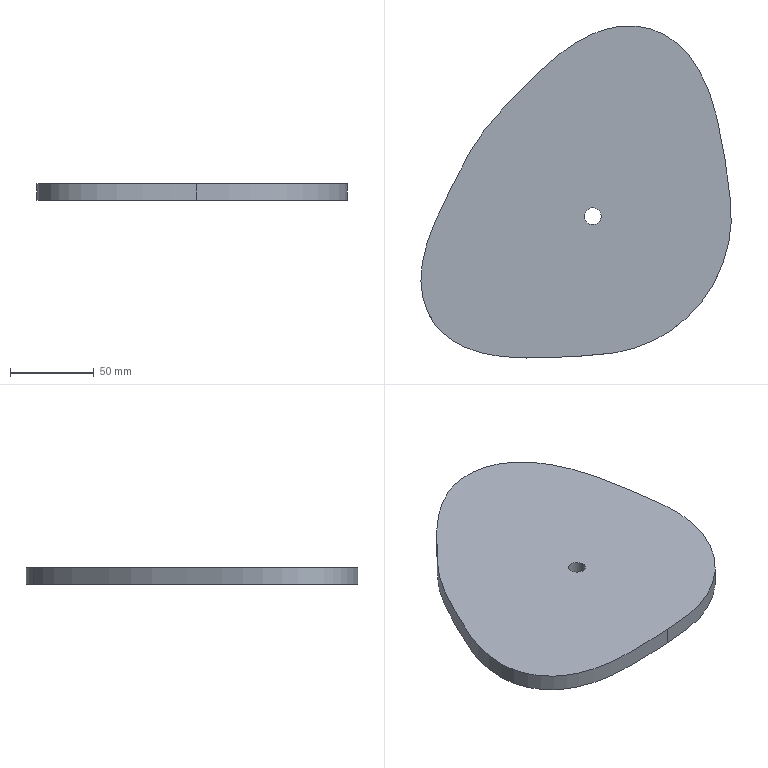Part | SolidWorks | features Extrusion 1 | 1 solid | 6 faces | box 185.51 x 198.55 x 10 mm | volume 275088 mm3 | cylinder 2 | plane 2 | spline 2 | commonest cylinder face diameters 10 x2
STEP:
#1=CARTESIAN_POINT('',(-5.,0.,10.));
#2=VERTEX_POINT('',#1);
#3=CARTESIAN_POINT('',(5.,0.,10.));
#4=VERTEX_POINT('',#3);
#5=CARTESIAN_POINT('',(0.,0.,10.));
#6=DIRECTION('',(0.,0.,1.));
#7=DIRECTION('',(1.,0.,0.));
#8=AXIS2_PLACEMENT_3D('',#5,#6,#7);
#9=CIRCLE('',#8,5.);
#10=EDGE_CURVE('',#2,#4,#9,.T.);
#11=ORIENTED_EDGE('',*,*,#10,.T.);
#12=CARTESIAN_POINT('',(5.,0.,0.));
#13=VERTEX_POINT('',#12);
#14=CARTESIAN_POINT('',(5.,0.,10.));
#15=DIRECTION('',(0.,0.,-1.));
#16=VECTOR('',#15,1000.);
#17=LINE('',#14,#16);
#18=EDGE_CURVE('',#4,#13,#17,.T.);
#19=ORIENTED_EDGE('',*,*,#18,.T.);
#20=CARTESIAN_POINT('',(-5.,0.,0.));
#21=VERTEX_POINT('',#20);
#22=CARTESIAN_POINT('',(0.,0.,0.));
#23=DIRECTION('',(0.,0.,1.));
#24=DIRECTION('',(1.,0.,0.));
#25=AXIS2_PLACEMENT_3D('',#22,#23,#24);
#26=CIRCLE('',#25,5.);
#27=EDGE_CURVE('',#21,#13,#26,.T.);
#28=ORIENTED_EDGE('',*,*,#27,.F.);
#29=CARTESIAN_POINT('',(-5.,0.,10.));
#30=DIRECTION('',(0.,0.,-1.));
#31=VECTOR('',#30,1000.);
#32=LINE('',#29,#31);
#33=EDGE_CURVE('',#2,#21,#32,.T.);
#34=ORIENTED_EDGE('',*,*,#33,.F.);
#35=EDGE_LOOP('',(#11,#19,#28,#34));
#36=FACE_OUTER_BOUND('',#35,.T.);
#37=CARTESIAN_POINT('',(0.,0.,10.));
#38=DIRECTION('',(0.,0.,-1.));
#39=DIRECTION('',(-1.,0.,0.));
#40=AXIS2_PLACEMENT_3D('',#37,#38,#39);
#41=CYLINDRICAL_SURFACE('',#40,5.);
#42=ADVANCED_FACE('',(#36),#41,.F.);
#43=CARTESIAN_POINT('',(-7.273,-83.589,10.));
#44=VERTEX_POINT('',#43);
#45=CARTESIAN_POINT('',(0.,109.019,10.));
#46=VERTEX_POINT('',#45);
#47=CARTESIAN_POINT('',(-7.273,-83.589,10.));
#48=CARTESIAN_POINT('',(-2.163,-83.305,10.));
#49=CARTESIAN_POINT('',(8.193,-82.677,10.));
#50=CARTESIAN_POINT('',(23.012,-79.954,10.));
#51=CARTESIAN_POINT('',(37.592,-74.228,10.));
#52=CARTESIAN_POINT('',(50.565,-66.119,10.));
#53=CARTESIAN_POINT('',(62.524,-54.944,10.));
#54=CARTESIAN_POINT('',(70.999,-43.258,10.));
#55=CARTESIAN_POINT('',(77.295,-30.405,10.));
#56=CARTESIAN_POINT('',(81.242,-17.641,10.));
#57=CARTESIAN_POINT('',(83.102,-3.246,10.));
#58=CARTESIAN_POINT('',(82.36,10.438,10.));
#59=CARTESIAN_POINT('',(80.506,24.371,10.));
#60=CARTESIAN_POINT('',(78.373,37.876,10.));
#61=CARTESIAN_POINT('',(75.984,51.161,10.));
#62=CARTESIAN_POINT('',(73.052,63.933,10.));
#63=CARTESIAN_POINT('',(69.233,75.903,10.));
#64=CARTESIAN_POINT('',(64.076,86.847,10.));
#65=CARTESIAN_POINT('',(58.392,95.36,10.));
#66=CARTESIAN_POINT('',(52.018,102.263,10.));
#67=CARTESIAN_POINT('',(44.725,107.796,10.));
#68=CARTESIAN_POINT('',(36.336,111.753,10.));
#69=CARTESIAN_POINT('',(27.254,113.834,10.));
#70=CARTESIAN_POINT('',(17.777,113.959,10.));
#71=CARTESIAN_POINT('',(8.517,112.296,10.));
#72=CARTESIAN_POINT('',(2.706,110.1,10.));
#73=CARTESIAN_POINT('',(0.,109.019,10.));
#74=B_SPLINE_CURVE_WITH_KNOTS('',3,(#47,#48,#49,#50,#51,#52,#53,#54,#55,#56,#57,#58,#59,#60,#61,#62,#63,#64,#65,#66,#67,#68,#69,#70,#71,#72,#73),.UNSPECIFIED.,.F.,.F.,(4,1,1,1,1,1,1,1,1,1,1,1,1,1,1,1,1,1,1,1,1,1,1,1,4),(0.,15.366,31.143,44.999,62.164,76.74,93.906,105.168,119.6,133.817,148.507,160.6,176.027,189.551,201.122,215.358,227.187,237.33,245.967,255.286,264.639,273.598,283.054,292.907,301.656),.UNSPECIFIED.);
#75=EDGE_CURVE('',#44,#46,#74,.T.);
#76=ORIENTED_EDGE('',*,*,#75,.T.);
#77=CARTESIAN_POINT('',(0.,109.019,10.));
#78=CARTESIAN_POINT('',(-1.743,108.323,10.));
#79=CARTESIAN_POINT('',(-7.298,105.557,10.));
#80=CARTESIAN_POINT('',(-18.846,98.358,10.));
#81=CARTESIAN_POINT('',(-32.919,85.931,10.));
#82=CARTESIAN_POINT('',(-48.133,70.236,10.));
#83=CARTESIAN_POINT('',(-61.72,56.014,10.));
#84=CARTESIAN_POINT('',(-72.325,41.044,10.));
#85=CARTESIAN_POINT('',(-79.964,26.234,10.));
#86=CARTESIAN_POINT('',(-87.981,10.6,10.));
#87=CARTESIAN_POINT('',(-95.298,-4.775,10.));
#88=CARTESIAN_POINT('',(-100.356,-19.035,10.));
#89=CARTESIAN_POINT('',(-102.796,-31.615,10.));
#90=CARTESIAN_POINT('',(-102.971,-43.123,10.));
#91=CARTESIAN_POINT('',(-100.703,-53.689,10.));
#92=CARTESIAN_POINT('',(-95.884,-63.296,10.));
#93=CARTESIAN_POINT('',(-89.114,-70.824,10.));
#94=CARTESIAN_POINT('',(-79.75,-77.203,10.));
#95=CARTESIAN_POINT('',(-68.146,-81.766,10.));
#96=CARTESIAN_POINT('',(-54.739,-84.163,10.));
#97=CARTESIAN_POINT('',(-39.991,-84.917,10.));
#98=CARTESIAN_POINT('',(-24.325,-84.473,10.));
#99=CARTESIAN_POINT('',(-12.978,-83.906,10.));
#100=CARTESIAN_POINT('',(-7.273,-83.589,10.));
#101=B_SPLINE_CURVE_WITH_KNOTS('',3,(#77,#78,#79,#80,#81,#82,#83,#84,#85,#86,#87,#88,#89,#90,#91,#92,#93,#94,#95,#96,#97,#98,#99,#100),.UNSPECIFIED.,.F.,.F.,(4,1,1,1,1,1,1,1,1,1,1,1,1,1,1,1,1,1,1,1,1,4),(301.656,307.291,320.251,342.406,363.41,385.94,401.355,418.297,435.908,454.133,469.385,481.202,492.455,503.723,513.291,524.418,533.709,547.101,561.508,574.423,591.384,608.539),.UNSPECIFIED.);
#102=EDGE_CURVE('',#46,#44,#101,.T.);
#103=ORIENTED_EDGE('',*,*,#102,.T.);
#104=EDGE_LOOP('',(#76,#103));
#105=FACE_OUTER_BOUND('',#104,.T.);
#106=ORIENTED_EDGE('',*,*,#10,.F.);
#107=CARTESIAN_POINT('',(0.,0.,10.));
#108=DIRECTION('',(0.,0.,1.));
#109=DIRECTION('',(1.,0.,0.));
#110=AXIS2_PLACEMENT_3D('',#107,#108,#109);
#111=CIRCLE('',#110,5.);
#112=EDGE_CURVE('',#4,#2,#111,.T.);
#113=ORIENTED_EDGE('',*,*,#112,.F.);
#114=EDGE_LOOP('',(#106,#113));
#115=FACE_BOUND('',#114,.T.);
#116=CARTESIAN_POINT('',(81.865,13.583,10.));
#117=DIRECTION('',(0.,0.,1.));
#118=DIRECTION('',(1.,0.,0.));
#119=AXIS2_PLACEMENT_3D('',#116,#117,#118);
#120=PLANE('',#119);
#121=ADVANCED_FACE('',(#105,#115),#120,.T.);
#122=CARTESIAN_POINT('',(-7.273,-83.589,0.));
#123=VERTEX_POINT('',#122);
#124=CARTESIAN_POINT('',(0.,109.019,0.));
#125=VERTEX_POINT('',#124);
#126=CARTESIAN_POINT('',(-7.273,-83.589,0.));
#127=CARTESIAN_POINT('',(-2.163,-83.305,0.));
#128=CARTESIAN_POINT('',(8.193,-82.677,0.));
#129=CARTESIAN_POINT('',(23.012,-79.954,0.));
#130=CARTESIAN_POINT('',(37.592,-74.228,0.));
#131=CARTESIAN_POINT('',(50.565,-66.119,0.));
#132=CARTESIAN_POINT('',(62.524,-54.944,0.));
#133=CARTESIAN_POINT('',(70.999,-43.258,0.));
#134=CARTESIAN_POINT('',(77.295,-30.405,0.));
#135=CARTESIAN_POINT('',(81.242,-17.641,0.));
#136=CARTESIAN_POINT('',(83.102,-3.246,0.));
#137=CARTESIAN_POINT('',(82.36,10.438,0.));
#138=CARTESIAN_POINT('',(80.506,24.371,0.));
#139=CARTESIAN_POINT('',(78.373,37.876,0.));
#140=CARTESIAN_POINT('',(75.984,51.161,0.));
#141=CARTESIAN_POINT('',(73.052,63.933,0.));
#142=CARTESIAN_POINT('',(69.233,75.903,0.));
#143=CARTESIAN_POINT('',(64.076,86.847,0.));
#144=CARTESIAN_POINT('',(58.392,95.36,0.));
#145=CARTESIAN_POINT('',(52.018,102.263,0.));
#146=CARTESIAN_POINT('',(44.725,107.796,0.));
#147=CARTESIAN_POINT('',(36.336,111.753,0.));
#148=CARTESIAN_POINT('',(27.254,113.834,0.));
#149=CARTESIAN_POINT('',(17.777,113.959,0.));
#150=CARTESIAN_POINT('',(8.517,112.296,0.));
#151=CARTESIAN_POINT('',(2.706,110.1,0.));
#152=CARTESIAN_POINT('',(0.,109.019,0.));
#153=B_SPLINE_CURVE_WITH_KNOTS('',3,(#126,#127,#128,#129,#130,#131,#132,#133,#134,#135,#136,#137,#138,#139,#140,#141,#142,#143,#144,#145,#146,#147,#148,#149,#150,#151,#152),.UNSPECIFIED.,.F.,.F.,(4,1,1,1,1,1,1,1,1,1,1,1,1,1,1,1,1,1,1,1,1,1,1,1,4),(0.,15.366,31.143,44.999,62.164,76.74,93.906,105.168,119.6,133.817,148.507,160.6,176.027,189.551,201.122,215.358,227.187,237.33,245.967,255.286,264.639,273.598,283.054,292.907,301.656),.UNSPECIFIED.);
#154=EDGE_CURVE('',#123,#125,#153,.T.);
#155=ORIENTED_EDGE('',*,*,#154,.F.);
#156=CARTESIAN_POINT('',(0.,109.019,0.));
#157=CARTESIAN_POINT('',(-1.743,108.323,0.));
#158=CARTESIAN_POINT('',(-7.298,105.557,0.));
#159=CARTESIAN_POINT('',(-18.846,98.358,0.));
#160=CARTESIAN_POINT('',(-32.919,85.931,0.));
#161=CARTESIAN_POINT('',(-48.133,70.236,0.));
#162=CARTESIAN_POINT('',(-61.72,56.014,0.));
#163=CARTESIAN_POINT('',(-72.325,41.044,0.));
#164=CARTESIAN_POINT('',(-79.964,26.234,0.));
#165=CARTESIAN_POINT('',(-87.981,10.6,0.));
#166=CARTESIAN_POINT('',(-95.298,-4.775,0.));
#167=CARTESIAN_POINT('',(-100.356,-19.035,0.));
#168=CARTESIAN_POINT('',(-102.796,-31.615,0.));
#169=CARTESIAN_POINT('',(-102.971,-43.123,0.));
#170=CARTESIAN_POINT('',(-100.703,-53.689,0.));
#171=CARTESIAN_POINT('',(-95.884,-63.296,0.));
#172=CARTESIAN_POINT('',(-89.114,-70.824,0.));
#173=CARTESIAN_POINT('',(-79.75,-77.203,0.));
#174=CARTESIAN_POINT('',(-68.146,-81.766,0.));
#175=CARTESIAN_POINT('',(-54.739,-84.163,0.));
#176=CARTESIAN_POINT('',(-39.991,-84.917,0.));
#177=CARTESIAN_POINT('',(-24.325,-84.473,0.));
#178=CARTESIAN_POINT('',(-12.978,-83.906,0.));
#179=CARTESIAN_POINT('',(-7.273,-83.589,0.));
#180=B_SPLINE_CURVE_WITH_KNOTS('',3,(#156,#157,#158,#159,#160,#161,#162,#163,#164,#165,#166,#167,#168,#169,#170,#171,#172,#173,#174,#175,#176,#177,#178,#179),.UNSPECIFIED.,.F.,.F.,(4,1,1,1,1,1,1,1,1,1,1,1,1,1,1,1,1,1,1,1,1,4),(301.656,307.291,320.251,342.406,363.41,385.94,401.355,418.297,435.908,454.133,469.385,481.202,492.455,503.723,513.291,524.418,533.709,547.101,561.508,574.423,591.384,608.539),.UNSPECIFIED.);
#181=EDGE_CURVE('',#125,#123,#180,.T.);
#182=ORIENTED_EDGE('',*,*,#181,.F.);
#183=EDGE_LOOP('',(#155,#182));
#184=FACE_OUTER_BOUND('',#183,.T.);
#185=ORIENTED_EDGE('',*,*,#27,.T.);
#186=CARTESIAN_POINT('',(0.,0.,0.));
#187=DIRECTION('',(0.,0.,1.));
#188=DIRECTION('',(1.,0.,0.));
#189=AXIS2_PLACEMENT_3D('',#186,#187,#188);
#190=CIRCLE('',#189,5.);
#191=EDGE_CURVE('',#13,#21,#190,.T.);
#192=ORIENTED_EDGE('',*,*,#191,.T.);
#193=EDGE_LOOP('',(#185,#192));
#194=FACE_BOUND('',#193,.T.);
#195=CARTESIAN_POINT('',(81.865,13.583,0.));
#196=DIRECTION('',(0.,0.,1.));
#197=DIRECTION('',(1.,0.,0.));
#198=AXIS2_PLACEMENT_3D('',#195,#196,#197);
#199=PLANE('',#198);
#200=ADVANCED_FACE('',(#184,#194),#199,.F.);
#201=ORIENTED_EDGE('',*,*,#154,.T.);
#202=CARTESIAN_POINT('',(0.,109.019,10.));
#203=DIRECTION('',(0.,0.,-1.));
#204=VECTOR('',#203,1000.);
#205=LINE('',#202,#204);
#206=EDGE_CURVE('',#46,#125,#205,.T.);
#207=ORIENTED_EDGE('',*,*,#206,.F.);
#208=ORIENTED_EDGE('',*,*,#75,.F.);
#209=CARTESIAN_POINT('',(-7.273,-83.589,10.));
#210=DIRECTION('',(0.,0.,-1.));
#211=VECTOR('',#210,1000.);
#212=LINE('',#209,#211);
#213=EDGE_CURVE('',#44,#123,#212,.T.);
#214=ORIENTED_EDGE('',*,*,#213,.T.);
#215=EDGE_LOOP('',(#201,#207,#208,#214));
#216=FACE_OUTER_BOUND('',#215,.T.);
#217=CARTESIAN_POINT('',(-7.273,-83.589,10.));
#218=CARTESIAN_POINT('',(-7.273,-83.589,0.));
#219=CARTESIAN_POINT('',(-2.163,-83.305,10.));
#220=CARTESIAN_POINT('',(-2.163,-83.305,0.));
#221=CARTESIAN_POINT('',(8.193,-82.677,10.));
#222=CARTESIAN_POINT('',(8.193,-82.677,0.));
#223=CARTESIAN_POINT('',(23.012,-79.954,10.));
#224=CARTESIAN_POINT('',(23.012,-79.954,0.));
#225=CARTESIAN_POINT('',(37.592,-74.228,10.));
#226=CARTESIAN_POINT('',(37.592,-74.228,0.));
#227=CARTESIAN_POINT('',(50.565,-66.119,10.));
#228=CARTESIAN_POINT('',(50.565,-66.119,0.));
#229=CARTESIAN_POINT('',(62.524,-54.944,10.));
#230=CARTESIAN_POINT('',(62.524,-54.944,0.));
#231=CARTESIAN_POINT('',(70.999,-43.258,10.));
#232=CARTESIAN_POINT('',(70.999,-43.258,0.));
#233=CARTESIAN_POINT('',(77.295,-30.405,10.));
#234=CARTESIAN_POINT('',(77.295,-30.405,0.));
#235=CARTESIAN_POINT('',(81.242,-17.641,10.));
#236=CARTESIAN_POINT('',(81.242,-17.641,0.));
#237=CARTESIAN_POINT('',(83.102,-3.246,10.));
#238=CARTESIAN_POINT('',(83.102,-3.246,0.));
#239=CARTESIAN_POINT('',(82.36,10.438,10.));
#240=CARTESIAN_POINT('',(82.36,10.438,0.));
#241=CARTESIAN_POINT('',(80.506,24.371,10.));
#242=CARTESIAN_POINT('',(80.506,24.371,0.));
#243=CARTESIAN_POINT('',(78.373,37.876,10.));
#244=CARTESIAN_POINT('',(78.373,37.876,0.));
#245=CARTESIAN_POINT('',(75.984,51.161,10.));
#246=CARTESIAN_POINT('',(75.984,51.161,0.));
#247=CARTESIAN_POINT('',(73.052,63.933,10.));
#248=CARTESIAN_POINT('',(73.052,63.933,0.));
#249=CARTESIAN_POINT('',(69.233,75.903,10.));
#250=CARTESIAN_POINT('',(69.233,75.903,0.));
#251=CARTESIAN_POINT('',(64.076,86.847,10.));
#252=CARTESIAN_POINT('',(64.076,86.847,0.));
#253=CARTESIAN_POINT('',(58.392,95.36,10.));
#254=CARTESIAN_POINT('',(58.392,95.36,0.));
#255=CARTESIAN_POINT('',(52.018,102.263,10.));
#256=CARTESIAN_POINT('',(52.018,102.263,0.));
#257=CARTESIAN_POINT('',(44.725,107.796,10.));
#258=CARTESIAN_POINT('',(44.725,107.796,0.));
#259=CARTESIAN_POINT('',(36.336,111.753,10.));
#260=CARTESIAN_POINT('',(36.336,111.753,0.));
#261=CARTESIAN_POINT('',(27.254,113.834,10.));
#262=CARTESIAN_POINT('',(27.254,113.834,0.));
#263=CARTESIAN_POINT('',(17.777,113.959,10.));
#264=CARTESIAN_POINT('',(17.777,113.959,0.));
#265=CARTESIAN_POINT('',(8.517,112.296,10.));
#266=CARTESIAN_POINT('',(8.517,112.296,0.));
#267=CARTESIAN_POINT('',(2.706,110.1,10.));
#268=CARTESIAN_POINT('',(2.706,110.1,0.));
#269=CARTESIAN_POINT('',(0.,109.019,10.));
#270=CARTESIAN_POINT('',(0.,109.019,0.));
#271=B_SPLINE_SURFACE_WITH_KNOTS('',3,1,((#217,#218),(#219,#220),(#221,#222),(#223,#224),(#225,#226),(#227,#228),(#229,#230),(#231,#232),(#233,#234),(#235,#236),(#237,#238),(#239,#240),(#241,#242),(#243,#244),(#245,#246),(#247,#248),(#249,#250),(#251,#252),(#253,#254),(#255,#256),(#257,#258),(#259,#260),(#261,#262),(#263,#264),(#265,#266),(#267,#268),(#269,#270)),.UNSPECIFIED.,.F.,.F.,.F.,(4,1,1,1,1,1,1,1,1,1,1,1,1,1,1,1,1,1,1,1,1,1,1,1,4),(2,2),(0.,15.366,31.143,44.999,62.164,76.74,93.906,105.168,119.6,133.817,148.507,160.6,176.027,189.551,201.122,215.358,227.187,237.33,245.967,255.286,264.639,273.598,283.054,292.907,301.656),(0.,1.),.UNSPECIFIED.);
#272=ADVANCED_FACE('',(#216),#271,.F.);
#273=ORIENTED_EDGE('',*,*,#181,.T.);
#274=ORIENTED_EDGE('',*,*,#213,.F.);
#275=ORIENTED_EDGE('',*,*,#102,.F.);
#276=ORIENTED_EDGE('',*,*,#206,.T.);
#277=EDGE_LOOP('',(#273,#274,#275,#276));
#278=FACE_OUTER_BOUND('',#277,.T.);
#279=CARTESIAN_POINT('',(0.,109.019,10.));
#280=CARTESIAN_POINT('',(0.,109.019,0.));
#281=CARTESIAN_POINT('',(-1.743,108.323,10.));
#282=CARTESIAN_POINT('',(-1.743,108.323,0.));
#283=CARTESIAN_POINT('',(-7.298,105.557,10.));
#284=CARTESIAN_POINT('',(-7.298,105.557,0.));
#285=CARTESIAN_POINT('',(-18.846,98.358,10.));
#286=CARTESIAN_POINT('',(-18.846,98.358,0.));
#287=CARTESIAN_POINT('',(-32.919,85.931,10.));
#288=CARTESIAN_POINT('',(-32.919,85.931,0.));
#289=CARTESIAN_POINT('',(-48.133,70.236,10.));
#290=CARTESIAN_POINT('',(-48.133,70.236,0.));
#291=CARTESIAN_POINT('',(-61.72,56.014,10.));
#292=CARTESIAN_POINT('',(-61.72,56.014,0.));
#293=CARTESIAN_POINT('',(-72.325,41.044,10.));
#294=CARTESIAN_POINT('',(-72.325,41.044,0.));
#295=CARTESIAN_POINT('',(-79.964,26.234,10.));
#296=CARTESIAN_POINT('',(-79.964,26.234,0.));
#297=CARTESIAN_POINT('',(-87.981,10.6,10.));
#298=CARTESIAN_POINT('',(-87.981,10.6,0.));
#299=CARTESIAN_POINT('',(-95.298,-4.775,10.));
#300=CARTESIAN_POINT('',(-95.298,-4.775,0.));
#301=CARTESIAN_POINT('',(-100.356,-19.035,10.));
#302=CARTESIAN_POINT('',(-100.356,-19.035,0.));
#303=CARTESIAN_POINT('',(-102.796,-31.615,10.));
#304=CARTESIAN_POINT('',(-102.796,-31.615,0.));
#305=CARTESIAN_POINT('',(-102.971,-43.123,10.));
#306=CARTESIAN_POINT('',(-102.971,-43.123,0.));
#307=CARTESIAN_POINT('',(-100.703,-53.689,10.));
#308=CARTESIAN_POINT('',(-100.703,-53.689,0.));
#309=CARTESIAN_POINT('',(-95.884,-63.296,10.));
#310=CARTESIAN_POINT('',(-95.884,-63.296,0.));
#311=CARTESIAN_POINT('',(-89.114,-70.824,10.));
#312=CARTESIAN_POINT('',(-89.114,-70.824,0.));
#313=CARTESIAN_POINT('',(-79.75,-77.203,10.));
#314=CARTESIAN_POINT('',(-79.75,-77.203,0.));
#315=CARTESIAN_POINT('',(-68.146,-81.766,10.));
#316=CARTESIAN_POINT('',(-68.146,-81.766,0.));
#317=CARTESIAN_POINT('',(-54.739,-84.163,10.));
#318=CARTESIAN_POINT('',(-54.739,-84.163,0.));
#319=CARTESIAN_POINT('',(-39.991,-84.917,10.));
#320=CARTESIAN_POINT('',(-39.991,-84.917,0.));
#321=CARTESIAN_POINT('',(-24.325,-84.473,10.));
#322=CARTESIAN_POINT('',(-24.325,-84.473,0.));
#323=CARTESIAN_POINT('',(-12.978,-83.906,10.));
#324=CARTESIAN_POINT('',(-12.978,-83.906,0.));
#325=CARTESIAN_POINT('',(-7.273,-83.589,10.));
#326=CARTESIAN_POINT('',(-7.273,-83.589,0.));
#327=B_SPLINE_SURFACE_WITH_KNOTS('',3,1,((#279,#280),(#281,#282),(#283,#284),(#285,#286),(#287,#288),(#289,#290),(#291,#292),(#293,#294),(#295,#296),(#297,#298),(#299,#300),(#301,#302),(#303,#304),(#305,#306),(#307,#308),(#309,#310),(#311,#312),(#313,#314),(#315,#316),(#317,#318),(#319,#320),(#321,#322),(#323,#324),(#325,#326)),.UNSPECIFIED.,.F.,.F.,.F.,(4,1,1,1,1,1,1,1,1,1,1,1,1,1,1,1,1,1,1,1,1,4),(2,2),(301.656,307.291,320.251,342.406,363.41,385.94,401.355,418.297,435.908,454.133,469.385,481.202,492.455,503.723,513.291,524.418,533.709,547.101,561.508,574.423,591.384,608.539),(0.,1.),.UNSPECIFIED.);
#328=ADVANCED_FACE('',(#278),#327,.F.);
#329=ORIENTED_EDGE('',*,*,#18,.F.);
#330=ORIENTED_EDGE('',*,*,#112,.T.);
#331=ORIENTED_EDGE('',*,*,#33,.T.);
#332=ORIENTED_EDGE('',*,*,#191,.F.);
#333=EDGE_LOOP('',(#329,#330,#331,#332));
#334=FACE_OUTER_BOUND('',#333,.T.);
#335=CARTESIAN_POINT('',(0.,0.,10.));
#336=DIRECTION('',(0.,0.,-1.));
#337=DIRECTION('',(-1.,0.,0.));
#338=AXIS2_PLACEMENT_3D('',#335,#336,#337);
#339=CYLINDRICAL_SURFACE('',#338,5.);
#340=ADVANCED_FACE('',(#334),#339,.F.);
#341=CLOSED_SHELL('',(#42,#121,#200,#272,#328,#340));
#342=MANIFOLD_SOLID_BREP('',#341);
#343=CARTESIAN_POINT('',(0.,0.,0.));
#344=DIRECTION('',(0.,0.,1.));
#345=DIRECTION('',(1.,0.,0.));
#346=AXIS2_PLACEMENT_3D('',#343,#344,#345);
#347=(LENGTH_UNIT()NAMED_UNIT(*)SI_UNIT(.MILLI.,.METRE.));
#348=UNCERTAINTY_MEASURE_WITH_UNIT(LENGTH_MEASURE(0.00001),#347,'','');
#349=(NAMED_UNIT(*)PLANE_ANGLE_UNIT()SI_UNIT($,.RADIAN.));
#350=(NAMED_UNIT(*)SI_UNIT($,.STERADIAN.)SOLID_ANGLE_UNIT());
#351=(GEOMETRIC_REPRESENTATION_CONTEXT(3)GLOBAL_UNCERTAINTY_ASSIGNED_CONTEXT((#348))GLOBAL_UNIT_ASSIGNED_CONTEXT((#347,#349,#350))REPRESENTATION_CONTEXT('',''));
#352=ADVANCED_BREP_SHAPE_REPRESENTATION('',(#342,#346),#351);